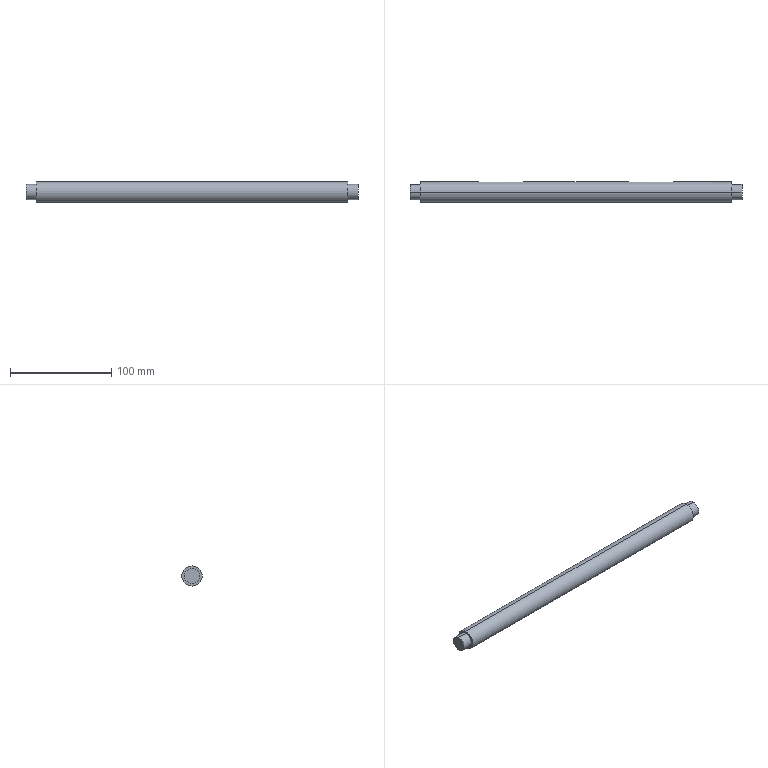Part | STEP file | PN_0032 (secondary rotating shaft) | 1 solid | 20 faces | box 328 x 20 x 20 mm | volume 99023 mm3 | cylinder 10 | plane 10 | commonest cylinder face diameters 5 x4 15 x4 20 x2